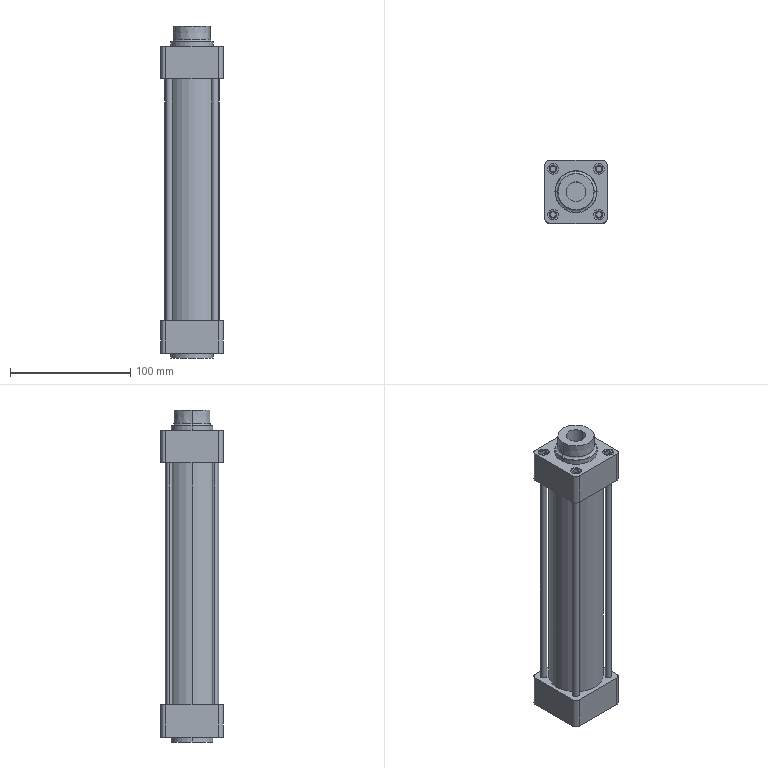Part | STEP file | 1 solid | 236 faces | box 52 x 52 x 276 mm | volume 460651 mm3 | plane 144 | cylinder 64 | cone 26 | torus 2 | commonest cylinder face diameters 4.773 x16 9 x16 5.3 x8 8 x8 7.8 x4 11.445 x4